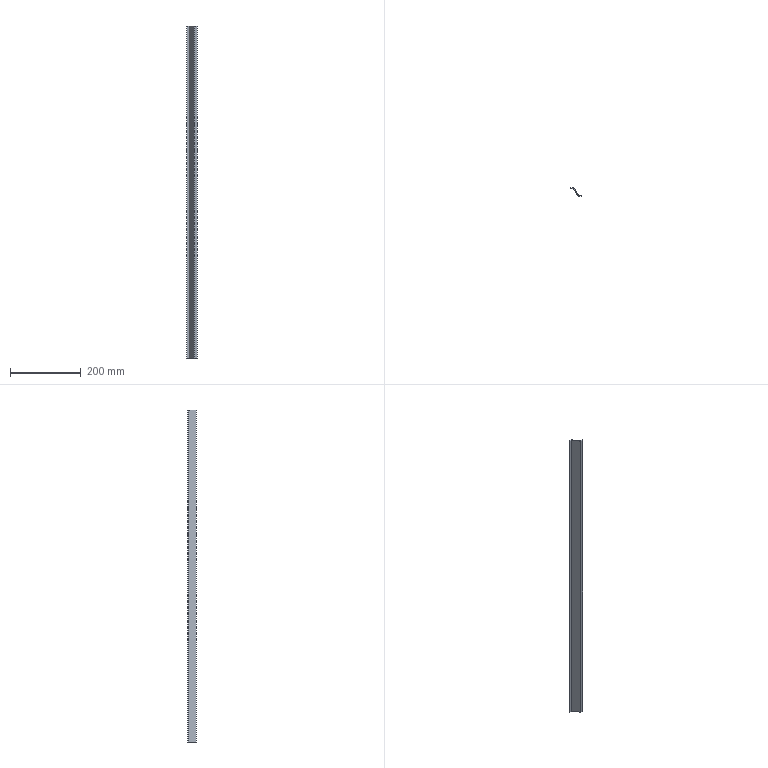Part | SolidWorks | features FlatPattern 1, SMBaseFlange 1, SheetMetal 1 | 1 solid | 10 faces | box 30 x 23 x 940 mm | volume 58296 mm3 | plane 10
STEP:
#1=CARTESIAN_POINT('',(-6.569,11.509,0.));
#2=VERTEX_POINT('',#1);
#3=CARTESIAN_POINT('',(-14.569,11.509,0.));
#4=VERTEX_POINT('',#3);
#5=CARTESIAN_POINT('',(-14.569,11.509,0.));
#6=DIRECTION('',(-1.,0.,0.));
#7=VECTOR('',#6,1000.);
#8=LINE('',#5,#7);
#9=EDGE_CURVE('',#2,#4,#8,.T.);
#10=ORIENTED_EDGE('',*,*,#9,.F.);
#11=CARTESIAN_POINT('',(-6.569,11.509,-940.));
#12=VERTEX_POINT('',#11);
#13=CARTESIAN_POINT('',(-6.569,11.509,-940.));
#14=DIRECTION('',(0.,0.,1.));
#15=VECTOR('',#14,1000.);
#16=LINE('',#13,#15);
#17=EDGE_CURVE('',#12,#2,#16,.T.);
#18=ORIENTED_EDGE('',*,*,#17,.F.);
#19=CARTESIAN_POINT('',(-14.569,11.509,-940.));
#20=VERTEX_POINT('',#19);
#21=CARTESIAN_POINT('',(-14.569,11.509,-940.));
#22=DIRECTION('',(-1.,0.,0.));
#23=VECTOR('',#22,1000.);
#24=LINE('',#21,#23);
#25=EDGE_CURVE('',#12,#20,#24,.T.);
#26=ORIENTED_EDGE('',*,*,#25,.T.);
#27=CARTESIAN_POINT('',(-14.569,11.509,-940.));
#28=DIRECTION('',(0.,0.,1.));
#29=VECTOR('',#28,1000.);
#30=LINE('',#27,#29);
#31=EDGE_CURVE('',#20,#4,#30,.T.);
#32=ORIENTED_EDGE('',*,*,#31,.T.);
#33=EDGE_LOOP('',(#10,#18,#26,#32));
#34=FACE_OUTER_BOUND('',#33,.T.);
#35=CARTESIAN_POINT('',(-14.569,11.509,-940.));
#36=DIRECTION('',(0.,1.,0.));
#37=DIRECTION('',(-1.,0.,0.));
#38=AXIS2_PLACEMENT_3D('',#35,#36,#37);
#39=PLANE('',#38);
#40=ADVANCED_FACE('',(#34),#39,.T.);
#41=CARTESIAN_POINT('',(8.222,-9.991,0.));
#42=VERTEX_POINT('',#41);
#43=CARTESIAN_POINT('',(-6.569,11.509,0.));
#44=DIRECTION('',(-0.5668,0.8239,0.));
#45=VECTOR('',#44,1000.);
#46=LINE('',#43,#45);
#47=EDGE_CURVE('',#42,#2,#46,.T.);
#48=ORIENTED_EDGE('',*,*,#47,.F.);
#49=CARTESIAN_POINT('',(8.222,-9.991,-940.));
#50=VERTEX_POINT('',#49);
#51=CARTESIAN_POINT('',(8.222,-9.991,-940.));
#52=DIRECTION('',(0.,0.,1.));
#53=VECTOR('',#52,1000.);
#54=LINE('',#51,#53);
#55=EDGE_CURVE('',#50,#42,#54,.T.);
#56=ORIENTED_EDGE('',*,*,#55,.F.);
#57=CARTESIAN_POINT('',(-6.569,11.509,-940.));
#58=DIRECTION('',(-0.5668,0.8239,0.));
#59=VECTOR('',#58,1000.);
#60=LINE('',#57,#59);
#61=EDGE_CURVE('',#50,#12,#60,.T.);
#62=ORIENTED_EDGE('',*,*,#61,.T.);
#63=ORIENTED_EDGE('',*,*,#17,.T.);
#64=EDGE_LOOP('',(#48,#56,#62,#63));
#65=FACE_OUTER_BOUND('',#64,.T.);
#66=CARTESIAN_POINT('',(-6.569,11.509,-940.));
#67=DIRECTION('',(0.8239,0.5668,0.));
#68=DIRECTION('',(-0.5668,0.8239,0.));
#69=AXIS2_PLACEMENT_3D('',#66,#67,#68);
#70=PLANE('',#69);
#71=ADVANCED_FACE('',(#65),#70,.T.);
#72=CARTESIAN_POINT('',(15.431,-9.991,0.));
#73=VERTEX_POINT('',#72);
#74=CARTESIAN_POINT('',(15.431,-9.991,0.));
#75=DIRECTION('',(-1.,0.,0.));
#76=VECTOR('',#75,1000.);
#77=LINE('',#74,#76);
#78=EDGE_CURVE('',#73,#42,#77,.T.);
#79=ORIENTED_EDGE('',*,*,#78,.F.);
#80=CARTESIAN_POINT('',(15.431,-9.991,-940.));
#81=VERTEX_POINT('',#80);
#82=CARTESIAN_POINT('',(15.431,-9.991,-940.));
#83=DIRECTION('',(0.,0.,1.));
#84=VECTOR('',#83,1000.);
#85=LINE('',#82,#84);
#86=EDGE_CURVE('',#81,#73,#85,.T.);
#87=ORIENTED_EDGE('',*,*,#86,.F.);
#88=CARTESIAN_POINT('',(15.431,-9.991,-940.));
#89=DIRECTION('',(-1.,0.,0.));
#90=VECTOR('',#89,1000.);
#91=LINE('',#88,#90);
#92=EDGE_CURVE('',#81,#50,#91,.T.);
#93=ORIENTED_EDGE('',*,*,#92,.T.);
#94=ORIENTED_EDGE('',*,*,#55,.T.);
#95=EDGE_LOOP('',(#79,#87,#93,#94));
#96=FACE_OUTER_BOUND('',#95,.T.);
#97=CARTESIAN_POINT('',(15.431,-9.991,-940.));
#98=DIRECTION('',(0.,1.,0.));
#99=DIRECTION('',(-1.,0.,0.));
#100=AXIS2_PLACEMENT_3D('',#97,#98,#99);
#101=PLANE('',#100);
#102=ADVANCED_FACE('',(#96),#101,.T.);
#103=CARTESIAN_POINT('',(15.431,-11.491,0.));
#104=VERTEX_POINT('',#103);
#105=CARTESIAN_POINT('',(15.431,-9.991,0.));
#106=DIRECTION('',(0.,1.,0.));
#107=VECTOR('',#106,1000.);
#108=LINE('',#105,#107);
#109=EDGE_CURVE('',#104,#73,#108,.T.);
#110=ORIENTED_EDGE('',*,*,#109,.F.);
#111=CARTESIAN_POINT('',(15.431,-11.491,-940.));
#112=VERTEX_POINT('',#111);
#113=CARTESIAN_POINT('',(15.431,-11.491,-940.));
#114=DIRECTION('',(0.,0.,1.));
#115=VECTOR('',#114,1000.);
#116=LINE('',#113,#115);
#117=EDGE_CURVE('',#112,#104,#116,.T.);
#118=ORIENTED_EDGE('',*,*,#117,.F.);
#119=CARTESIAN_POINT('',(15.431,-9.991,-940.));
#120=DIRECTION('',(0.,1.,0.));
#121=VECTOR('',#120,1000.);
#122=LINE('',#119,#121);
#123=EDGE_CURVE('',#112,#81,#122,.T.);
#124=ORIENTED_EDGE('',*,*,#123,.T.);
#125=ORIENTED_EDGE('',*,*,#86,.T.);
#126=EDGE_LOOP('',(#110,#118,#124,#125));
#127=FACE_OUTER_BOUND('',#126,.T.);
#128=CARTESIAN_POINT('',(15.431,-9.991,-940.));
#129=DIRECTION('',(1.,0.,0.));
#130=DIRECTION('',(0.,1.,0.));
#131=AXIS2_PLACEMENT_3D('',#128,#129,#130);
#132=PLANE('',#131);
#133=ADVANCED_FACE('',(#127),#132,.T.);
#134=CARTESIAN_POINT('',(7.431,-11.491,0.));
#135=VERTEX_POINT('',#134);
#136=CARTESIAN_POINT('',(15.431,-11.491,0.));
#137=DIRECTION('',(1.,0.,0.));
#138=VECTOR('',#137,1000.);
#139=LINE('',#136,#138);
#140=EDGE_CURVE('',#135,#104,#139,.T.);
#141=ORIENTED_EDGE('',*,*,#140,.F.);
#142=CARTESIAN_POINT('',(7.431,-11.491,-940.));
#143=VERTEX_POINT('',#142);
#144=CARTESIAN_POINT('',(7.431,-11.491,-940.));
#145=DIRECTION('',(0.,0.,1.));
#146=VECTOR('',#145,1000.);
#147=LINE('',#144,#146);
#148=EDGE_CURVE('',#143,#135,#147,.T.);
#149=ORIENTED_EDGE('',*,*,#148,.F.);
#150=CARTESIAN_POINT('',(15.431,-11.491,-940.));
#151=DIRECTION('',(1.,0.,0.));
#152=VECTOR('',#151,1000.);
#153=LINE('',#150,#152);
#154=EDGE_CURVE('',#143,#112,#153,.T.);
#155=ORIENTED_EDGE('',*,*,#154,.T.);
#156=ORIENTED_EDGE('',*,*,#117,.T.);
#157=EDGE_LOOP('',(#141,#149,#155,#156));
#158=FACE_OUTER_BOUND('',#157,.T.);
#159=CARTESIAN_POINT('',(15.431,-11.491,-940.));
#160=DIRECTION('',(0.,-1.,0.));
#161=DIRECTION('',(0.,0.,-1.));
#162=AXIS2_PLACEMENT_3D('',#159,#160,#161);
#163=PLANE('',#162);
#164=ADVANCED_FACE('',(#158),#163,.T.);
#165=CARTESIAN_POINT('',(-7.361,10.009,0.));
#166=VERTEX_POINT('',#165);
#167=CARTESIAN_POINT('',(-7.361,10.009,0.));
#168=DIRECTION('',(0.5668,-0.8239,0.));
#169=VECTOR('',#168,1000.);
#170=LINE('',#167,#169);
#171=EDGE_CURVE('',#166,#135,#170,.T.);
#172=ORIENTED_EDGE('',*,*,#171,.F.);
#173=CARTESIAN_POINT('',(-7.361,10.009,-940.));
#174=VERTEX_POINT('',#173);
#175=CARTESIAN_POINT('',(-7.361,10.009,-940.));
#176=DIRECTION('',(0.,0.,1.));
#177=VECTOR('',#176,1000.);
#178=LINE('',#175,#177);
#179=EDGE_CURVE('',#174,#166,#178,.T.);
#180=ORIENTED_EDGE('',*,*,#179,.F.);
#181=CARTESIAN_POINT('',(-7.361,10.009,-940.));
#182=DIRECTION('',(0.5668,-0.8239,0.));
#183=VECTOR('',#182,1000.);
#184=LINE('',#181,#183);
#185=EDGE_CURVE('',#174,#143,#184,.T.);
#186=ORIENTED_EDGE('',*,*,#185,.T.);
#187=ORIENTED_EDGE('',*,*,#148,.T.);
#188=EDGE_LOOP('',(#172,#180,#186,#187));
#189=FACE_OUTER_BOUND('',#188,.T.);
#190=CARTESIAN_POINT('',(-7.361,10.009,-940.));
#191=DIRECTION('',(-0.8239,-0.5668,0.));
#192=DIRECTION('',(0.5668,-0.8239,0.));
#193=AXIS2_PLACEMENT_3D('',#190,#191,#192);
#194=PLANE('',#193);
#195=ADVANCED_FACE('',(#189),#194,.T.);
#196=CARTESIAN_POINT('',(-14.569,10.009,0.));
#197=VERTEX_POINT('',#196);
#198=CARTESIAN_POINT('',(-14.569,10.009,0.));
#199=DIRECTION('',(1.,0.,0.));
#200=VECTOR('',#199,1000.);
#201=LINE('',#198,#200);
#202=EDGE_CURVE('',#197,#166,#201,.T.);
#203=ORIENTED_EDGE('',*,*,#202,.F.);
#204=CARTESIAN_POINT('',(-14.569,10.009,-940.));
#205=VERTEX_POINT('',#204);
#206=CARTESIAN_POINT('',(-14.569,10.009,-940.));
#207=DIRECTION('',(0.,0.,1.));
#208=VECTOR('',#207,1000.);
#209=LINE('',#206,#208);
#210=EDGE_CURVE('',#205,#197,#209,.T.);
#211=ORIENTED_EDGE('',*,*,#210,.F.);
#212=CARTESIAN_POINT('',(-14.569,10.009,-940.));
#213=DIRECTION('',(1.,0.,0.));
#214=VECTOR('',#213,1000.);
#215=LINE('',#212,#214);
#216=EDGE_CURVE('',#205,#174,#215,.T.);
#217=ORIENTED_EDGE('',*,*,#216,.T.);
#218=ORIENTED_EDGE('',*,*,#179,.T.);
#219=EDGE_LOOP('',(#203,#211,#217,#218));
#220=FACE_OUTER_BOUND('',#219,.T.);
#221=CARTESIAN_POINT('',(-14.569,10.009,-940.));
#222=DIRECTION('',(0.,-1.,0.));
#223=DIRECTION('',(0.,0.,-1.));
#224=AXIS2_PLACEMENT_3D('',#221,#222,#223);
#225=PLANE('',#224);
#226=ADVANCED_FACE('',(#220),#225,.T.);
#227=CARTESIAN_POINT('',(-14.569,11.509,0.));
#228=DIRECTION('',(0.,-1.,0.));
#229=VECTOR('',#228,1000.);
#230=LINE('',#227,#229);
#231=EDGE_CURVE('',#4,#197,#230,.T.);
#232=ORIENTED_EDGE('',*,*,#231,.F.);
#233=ORIENTED_EDGE('',*,*,#31,.F.);
#234=CARTESIAN_POINT('',(-14.569,11.509,-940.));
#235=DIRECTION('',(0.,-1.,0.));
#236=VECTOR('',#235,1000.);
#237=LINE('',#234,#236);
#238=EDGE_CURVE('',#20,#205,#237,.T.);
#239=ORIENTED_EDGE('',*,*,#238,.T.);
#240=ORIENTED_EDGE('',*,*,#210,.T.);
#241=EDGE_LOOP('',(#232,#233,#239,#240));
#242=FACE_OUTER_BOUND('',#241,.T.);
#243=CARTESIAN_POINT('',(-14.569,11.509,-940.));
#244=DIRECTION('',(-1.,0.,0.));
#245=DIRECTION('',(0.,0.,1.));
#246=AXIS2_PLACEMENT_3D('',#243,#244,#245);
#247=PLANE('',#246);
#248=ADVANCED_FACE('',(#242),#247,.T.);
#249=ORIENTED_EDGE('',*,*,#25,.F.);
#250=ORIENTED_EDGE('',*,*,#61,.F.);
#251=ORIENTED_EDGE('',*,*,#92,.F.);
#252=ORIENTED_EDGE('',*,*,#123,.F.);
#253=ORIENTED_EDGE('',*,*,#154,.F.);
#254=ORIENTED_EDGE('',*,*,#185,.F.);
#255=ORIENTED_EDGE('',*,*,#216,.F.);
#256=ORIENTED_EDGE('',*,*,#238,.F.);
#257=EDGE_LOOP('',(#249,#250,#251,#252,#253,#254,#255,#256));
#258=FACE_OUTER_BOUND('',#257,.T.);
#259=CARTESIAN_POINT('',(0.,0.,-940.));
#260=DIRECTION('',(0.,0.,-1.));
#261=DIRECTION('',(-1.,0.,0.));
#262=AXIS2_PLACEMENT_3D('',#259,#260,#261);
#263=PLANE('',#262);
#264=ADVANCED_FACE('',(#258),#263,.T.);
#265=ORIENTED_EDGE('',*,*,#9,.T.);
#266=ORIENTED_EDGE('',*,*,#231,.T.);
#267=ORIENTED_EDGE('',*,*,#202,.T.);
#268=ORIENTED_EDGE('',*,*,#171,.T.);
#269=ORIENTED_EDGE('',*,*,#140,.T.);
#270=ORIENTED_EDGE('',*,*,#109,.T.);
#271=ORIENTED_EDGE('',*,*,#78,.T.);
#272=ORIENTED_EDGE('',*,*,#47,.T.);
#273=EDGE_LOOP('',(#265,#266,#267,#268,#269,#270,#271,#272));
#274=FACE_OUTER_BOUND('',#273,.T.);
#275=CARTESIAN_POINT('',(0.,0.,0.));
#276=DIRECTION('',(0.,0.,-1.));
#277=DIRECTION('',(-1.,0.,0.));
#278=AXIS2_PLACEMENT_3D('',#275,#276,#277);
#279=PLANE('',#278);
#280=ADVANCED_FACE('',(#274),#279,.F.);
#281=CLOSED_SHELL('',(#40,#71,#102,#133,#164,#195,#226,#248,#264,#280));
#282=MANIFOLD_SOLID_BREP('',#281);
#283=CARTESIAN_POINT('',(0.,0.,0.));
#284=DIRECTION('',(0.,0.,1.));
#285=DIRECTION('',(1.,0.,0.));
#286=AXIS2_PLACEMENT_3D('',#283,#284,#285);
#287=(LENGTH_UNIT()NAMED_UNIT(*)SI_UNIT(.MILLI.,.METRE.));
#288=UNCERTAINTY_MEASURE_WITH_UNIT(LENGTH_MEASURE(0.00001),#287,'','');
#289=(NAMED_UNIT(*)PLANE_ANGLE_UNIT()SI_UNIT($,.RADIAN.));
#290=(NAMED_UNIT(*)SI_UNIT($,.STERADIAN.)SOLID_ANGLE_UNIT());
#291=(GEOMETRIC_REPRESENTATION_CONTEXT(3)GLOBAL_UNCERTAINTY_ASSIGNED_CONTEXT((#288))GLOBAL_UNIT_ASSIGNED_CONTEXT((#287,#289,#290))REPRESENTATION_CONTEXT('',''));
#292=ADVANCED_BREP_SHAPE_REPRESENTATION('',(#282,#286),#291);